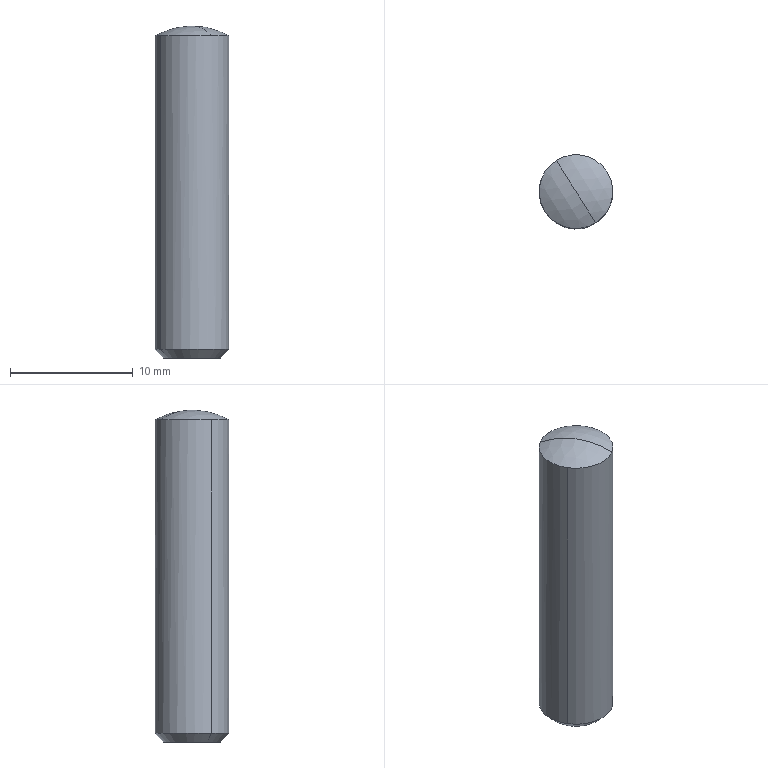Part | SolidWorks | features BaseBody 1 | 1 solid | 7 faces | box 6 x 6 x 27 mm | volume 748.056 mm3 | cone 2 | sphere 2 | cylinder 2 | plane 1 | commonest cylinder face diameters 6 x2
STEP:
#1=CARTESIAN_POINT('',(108.547,-22.215,39.5));
#2=VERTEX_POINT('',#1);
#3=CARTESIAN_POINT('',(112.453,-19.785,39.5));
#4=VERTEX_POINT('',#3);
#5=CARTESIAN_POINT('',(110.5,-21.,39.5));
#6=DIRECTION('',(0.,0.,-1.));
#7=DIRECTION('',(-0.8491,-0.5282,0.));
#8=AXIS2_PLACEMENT_3D('',#5,#6,#7);
#9=CIRCLE('',#8,2.3);
#10=EDGE_CURVE('',#2,#4,#9,.T.);
#11=ORIENTED_EDGE('',*,*,#10,.F.);
#12=CARTESIAN_POINT('',(107.953,-22.585,40.2));
#13=VERTEX_POINT('',#12);
#14=CARTESIAN_POINT('',(108.547,-22.215,39.5));
#15=DIRECTION('',(-0.6004,-0.3735,0.7071));
#16=VECTOR('',#15,1000.);
#17=LINE('',#14,#16);
#18=EDGE_CURVE('',#2,#13,#17,.T.);
#19=ORIENTED_EDGE('',*,*,#18,.T.);
#20=CARTESIAN_POINT('',(113.047,-19.415,40.2));
#21=VERTEX_POINT('',#20);
#22=CARTESIAN_POINT('',(110.5,-21.,40.2));
#23=DIRECTION('',(0.,0.,1.));
#24=DIRECTION('',(-0.8491,-0.5282,0.));
#25=AXIS2_PLACEMENT_3D('',#22,#23,#24);
#26=CIRCLE('',#25,3.);
#27=EDGE_CURVE('',#21,#13,#26,.T.);
#28=ORIENTED_EDGE('',*,*,#27,.F.);
#29=CARTESIAN_POINT('',(112.453,-19.785,39.5));
#30=DIRECTION('',(0.6004,0.3735,0.7071));
#31=VECTOR('',#30,1000.);
#32=LINE('',#29,#31);
#33=EDGE_CURVE('',#4,#21,#32,.T.);
#34=ORIENTED_EDGE('',*,*,#33,.F.);
#35=EDGE_LOOP('',(#11,#19,#28,#34));
#36=FACE_OUTER_BOUND('',#35,.T.);
#37=CARTESIAN_POINT('',(110.5,-21.,39.5));
#38=DIRECTION('',(0.,0.,1.));
#39=DIRECTION('',(0.8491,0.5282,0.));
#40=AXIS2_PLACEMENT_3D('',#37,#38,#39);
#41=CONICAL_SURFACE('',#40,2.3,0.7854);
#42=ADVANCED_FACE('',(#36),#41,.T.);
#43=CARTESIAN_POINT('',(110.5,-21.,66.5));
#44=VERTEX_POINT('',#43);
#45=CARTESIAN_POINT('',(108.915,-18.453,65.696));
#46=VERTEX_POINT('',#45);
#47=CARTESIAN_POINT('',(110.5,-21.,60.5));
#48=DIRECTION('',(-0.8491,-0.5282,0.));
#49=DIRECTION('',(0.5282,-0.8491,0.));
#50=AXIS2_PLACEMENT_3D('',#47,#48,#49);
#51=CIRCLE('',#50,6.);
#52=EDGE_CURVE('',#44,#46,#51,.T.);
#53=ORIENTED_EDGE('',*,*,#52,.F.);
#54=CARTESIAN_POINT('',(112.085,-23.547,65.696));
#55=VERTEX_POINT('',#54);
#56=CARTESIAN_POINT('',(110.5,-21.,60.5));
#57=DIRECTION('',(0.8491,0.5282,0.));
#58=DIRECTION('',(-0.5282,0.8491,0.));
#59=AXIS2_PLACEMENT_3D('',#56,#57,#58);
#60=CIRCLE('',#59,6.);
#61=EDGE_CURVE('',#44,#55,#60,.T.);
#62=ORIENTED_EDGE('',*,*,#61,.T.);
#63=CARTESIAN_POINT('',(113.047,-19.415,65.696));
#64=VERTEX_POINT('',#63);
#65=CARTESIAN_POINT('',(110.5,-21.,65.696));
#66=DIRECTION('',(0.,0.,-1.));
#67=DIRECTION('',(-0.8491,-0.5282,0.));
#68=AXIS2_PLACEMENT_3D('',#65,#66,#67);
#69=CIRCLE('',#68,3.);
#70=EDGE_CURVE('',#64,#55,#69,.T.);
#71=ORIENTED_EDGE('',*,*,#70,.F.);
#72=CARTESIAN_POINT('',(110.5,-21.,65.696));
#73=DIRECTION('',(0.,0.,-1.));
#74=DIRECTION('',(-0.8491,-0.5282,0.));
#75=AXIS2_PLACEMENT_3D('',#72,#73,#74);
#76=CIRCLE('',#75,3.);
#77=EDGE_CURVE('',#46,#64,#76,.T.);
#78=ORIENTED_EDGE('',*,*,#77,.F.);
#79=EDGE_LOOP('',(#53,#62,#71,#78));
#80=FACE_OUTER_BOUND('',#79,.T.);
#81=CARTESIAN_POINT('',(110.5,-21.,60.5));
#82=DIRECTION('',(0.8491,0.5282,0.));
#83=DIRECTION('',(-0.5282,0.8491,0.));
#84=AXIS2_PLACEMENT_3D('',#81,#82,#83);
#85=SPHERICAL_SURFACE('',#84,6.);
#86=ADVANCED_FACE('',(#80),#85,.T.);
#87=CARTESIAN_POINT('',(107.953,-22.585,65.696));
#88=VERTEX_POINT('',#87);
#89=CARTESIAN_POINT('',(110.5,-21.,65.696));
#90=DIRECTION('',(0.,0.,-1.));
#91=DIRECTION('',(-0.8491,-0.5282,0.));
#92=AXIS2_PLACEMENT_3D('',#89,#90,#91);
#93=CIRCLE('',#92,3.);
#94=EDGE_CURVE('',#88,#46,#93,.T.);
#95=ORIENTED_EDGE('',*,*,#94,.T.);
#96=ORIENTED_EDGE('',*,*,#77,.T.);
#97=CARTESIAN_POINT('',(113.047,-19.415,39.5));
#98=DIRECTION('',(0.,0.,-1.));
#99=VECTOR('',#98,1000.);
#100=LINE('',#97,#99);
#101=EDGE_CURVE('',#64,#21,#100,.T.);
#102=ORIENTED_EDGE('',*,*,#101,.T.);
#103=ORIENTED_EDGE('',*,*,#27,.T.);
#104=CARTESIAN_POINT('',(107.953,-22.585,39.5));
#105=DIRECTION('',(0.,0.,-1.));
#106=VECTOR('',#105,1000.);
#107=LINE('',#104,#106);
#108=EDGE_CURVE('',#88,#13,#107,.T.);
#109=ORIENTED_EDGE('',*,*,#108,.F.);
#110=EDGE_LOOP('',(#95,#96,#102,#103,#109));
#111=FACE_OUTER_BOUND('',#110,.T.);
#112=CARTESIAN_POINT('',(110.5,-21.,39.5));
#113=DIRECTION('',(0.,0.,-1.));
#114=DIRECTION('',(-0.8491,-0.5282,0.));
#115=AXIS2_PLACEMENT_3D('',#112,#113,#114);
#116=CYLINDRICAL_SURFACE('',#115,3.);
#117=ADVANCED_FACE('',(#111),#116,.T.);
#118=CARTESIAN_POINT('',(110.5,-21.,39.5));
#119=DIRECTION('',(0.,0.,-1.));
#120=DIRECTION('',(-0.8491,-0.5282,0.));
#121=AXIS2_PLACEMENT_3D('',#118,#119,#120);
#122=CIRCLE('',#121,2.3);
#123=EDGE_CURVE('',#4,#2,#122,.T.);
#124=ORIENTED_EDGE('',*,*,#123,.T.);
#125=ORIENTED_EDGE('',*,*,#10,.T.);
#126=EDGE_LOOP('',(#124,#125));
#127=FACE_OUTER_BOUND('',#126,.T.);
#128=CARTESIAN_POINT('',(110.5,-21.,39.5));
#129=DIRECTION('',(0.,0.,-1.));
#130=DIRECTION('',(-0.8491,-0.5282,0.));
#131=AXIS2_PLACEMENT_3D('',#128,#129,#130);
#132=PLANE('',#131);
#133=ADVANCED_FACE('',(#127),#132,.T.);
#134=ORIENTED_EDGE('',*,*,#101,.F.);
#135=ORIENTED_EDGE('',*,*,#70,.T.);
#136=CARTESIAN_POINT('',(110.5,-21.,65.696));
#137=DIRECTION('',(0.,0.,-1.));
#138=DIRECTION('',(-0.8491,-0.5282,0.));
#139=AXIS2_PLACEMENT_3D('',#136,#137,#138);
#140=CIRCLE('',#139,3.);
#141=EDGE_CURVE('',#55,#88,#140,.T.);
#142=ORIENTED_EDGE('',*,*,#141,.T.);
#143=ORIENTED_EDGE('',*,*,#108,.T.);
#144=CARTESIAN_POINT('',(110.5,-21.,40.2));
#145=DIRECTION('',(0.,0.,1.));
#146=DIRECTION('',(-0.8491,-0.5282,0.));
#147=AXIS2_PLACEMENT_3D('',#144,#145,#146);
#148=CIRCLE('',#147,3.);
#149=EDGE_CURVE('',#13,#21,#148,.T.);
#150=ORIENTED_EDGE('',*,*,#149,.T.);
#151=EDGE_LOOP('',(#134,#135,#142,#143,#150));
#152=FACE_OUTER_BOUND('',#151,.T.);
#153=CARTESIAN_POINT('',(110.5,-21.,39.5));
#154=DIRECTION('',(0.,0.,-1.));
#155=DIRECTION('',(-0.8491,-0.5282,0.));
#156=AXIS2_PLACEMENT_3D('',#153,#154,#155);
#157=CYLINDRICAL_SURFACE('',#156,3.);
#158=ADVANCED_FACE('',(#152),#157,.T.);
#159=ORIENTED_EDGE('',*,*,#61,.F.);
#160=ORIENTED_EDGE('',*,*,#52,.T.);
#161=ORIENTED_EDGE('',*,*,#94,.F.);
#162=ORIENTED_EDGE('',*,*,#141,.F.);
#163=EDGE_LOOP('',(#159,#160,#161,#162));
#164=FACE_OUTER_BOUND('',#163,.T.);
#165=CARTESIAN_POINT('',(110.5,-21.,60.5));
#166=DIRECTION('',(0.8491,0.5282,0.));
#167=DIRECTION('',(-0.5282,0.8491,0.));
#168=AXIS2_PLACEMENT_3D('',#165,#166,#167);
#169=SPHERICAL_SURFACE('',#168,6.);
#170=ADVANCED_FACE('',(#164),#169,.T.);
#171=ORIENTED_EDGE('',*,*,#18,.F.);
#172=ORIENTED_EDGE('',*,*,#123,.F.);
#173=ORIENTED_EDGE('',*,*,#33,.T.);
#174=ORIENTED_EDGE('',*,*,#149,.F.);
#175=EDGE_LOOP('',(#171,#172,#173,#174));
#176=FACE_OUTER_BOUND('',#175,.T.);
#177=CARTESIAN_POINT('',(110.5,-21.,39.5));
#178=DIRECTION('',(0.,0.,1.));
#179=DIRECTION('',(0.8491,0.5282,0.));
#180=AXIS2_PLACEMENT_3D('',#177,#178,#179);
#181=CONICAL_SURFACE('',#180,2.3,0.7854);
#182=ADVANCED_FACE('',(#176),#181,.T.);
#183=CLOSED_SHELL('',(#42,#86,#117,#133,#158,#170,#182));
#184=MANIFOLD_SOLID_BREP('',#183);
#185=CARTESIAN_POINT('',(0.,0.,0.));
#186=DIRECTION('',(0.,0.,1.));
#187=DIRECTION('',(1.,0.,0.));
#188=AXIS2_PLACEMENT_3D('',#185,#186,#187);
#189=(LENGTH_UNIT()NAMED_UNIT(*)SI_UNIT(.MILLI.,.METRE.));
#190=UNCERTAINTY_MEASURE_WITH_UNIT(LENGTH_MEASURE(0.00001),#189,'','');
#191=(NAMED_UNIT(*)PLANE_ANGLE_UNIT()SI_UNIT($,.RADIAN.));
#192=(NAMED_UNIT(*)SI_UNIT($,.STERADIAN.)SOLID_ANGLE_UNIT());
#193=(GEOMETRIC_REPRESENTATION_CONTEXT(3)GLOBAL_UNCERTAINTY_ASSIGNED_CONTEXT((#190))GLOBAL_UNIT_ASSIGNED_CONTEXT((#189,#191,#192))REPRESENTATION_CONTEXT('',''));
#194=ADVANCED_BREP_SHAPE_REPRESENTATION('',(#184,#188),#193);